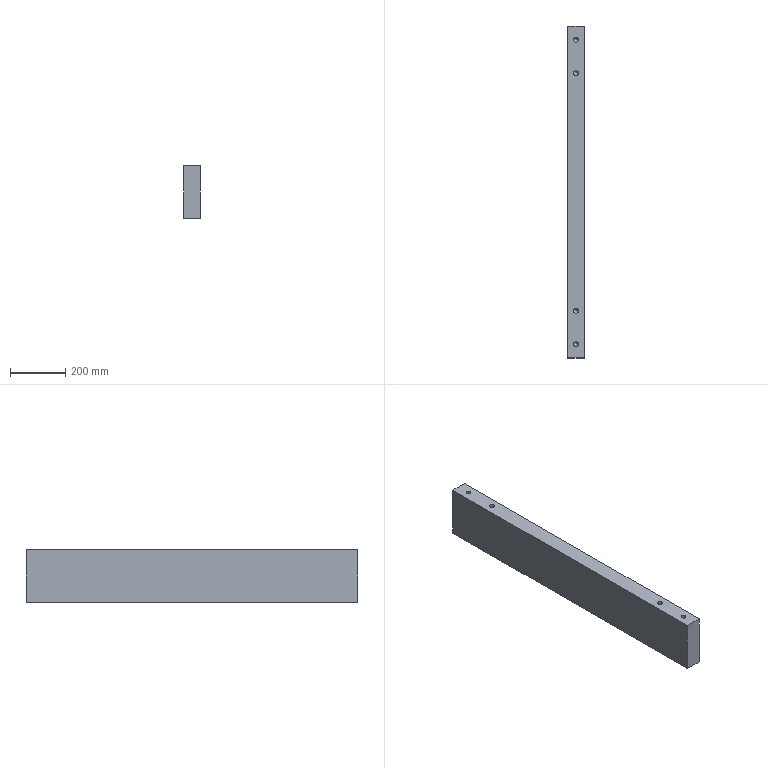Part | STEP file | lll_id4238_x_t | 1 solid | 22 faces | box 60 x 1200 x 190 mm | volume 13594949 mm3 | cylinder 8 | cone 8 | plane 6 | commonest cylinder face diameters 17.506 x7 17.505 x1
STEP:
#1=CARTESIAN_POINT('',(2996.188,-550.,-370.));
#2=VERTEX_POINT('',#1);
#3=CARTESIAN_POINT('',(2987.435,-550.,-370.));
#4=DIRECTION('',(0.,0.,1.));
#5=DIRECTION('',(1.,0.,0.));
#6=AXIS2_PLACEMENT_3D('',#3,#4,#5);
#7=CIRCLE('',#6,8.753);
#8=EDGE_CURVE('',#2,#2,#7,.T.);
#9=ORIENTED_EDGE('',*,*,#8,.T.);
#10=EDGE_LOOP('',(#9));
#11=FACE_BOUND('',#10,.T.);
#12=CARTESIAN_POINT('',(2996.188,550.,-370.));
#13=VERTEX_POINT('',#12);
#14=CARTESIAN_POINT('',(2987.435,550.,-370.));
#15=DIRECTION('',(0.,0.,1.));
#16=DIRECTION('',(1.,0.,0.));
#17=AXIS2_PLACEMENT_3D('',#14,#15,#16);
#18=CIRCLE('',#17,8.753);
#19=EDGE_CURVE('',#13,#13,#18,.T.);
#20=ORIENTED_EDGE('',*,*,#19,.T.);
#21=EDGE_LOOP('',(#20));
#22=FACE_BOUND('',#21,.T.);
#23=CARTESIAN_POINT('',(2957.435,600.,-370.));
#24=VERTEX_POINT('',#23);
#25=CARTESIAN_POINT('',(2957.435,-600.,-370.));
#26=VERTEX_POINT('',#25);
#27=CARTESIAN_POINT('',(2957.435,1.,-370.));
#28=DIRECTION('',(0.,-1.,0.));
#29=VECTOR('',#28,1.);
#30=LINE('',#27,#29);
#31=EDGE_CURVE('',#24,#26,#30,.T.);
#32=ORIENTED_EDGE('',*,*,#31,.F.);
#33=CARTESIAN_POINT('',(3017.435,600.,-370.));
#34=VERTEX_POINT('',#33);
#35=CARTESIAN_POINT('',(-952.565,600.,-370.));
#36=DIRECTION('',(1.,0.,0.));
#37=VECTOR('',#36,1.);
#38=LINE('',#35,#37);
#39=EDGE_CURVE('',#24,#34,#38,.T.);
#40=ORIENTED_EDGE('',*,*,#39,.T.);
#41=CARTESIAN_POINT('',(3017.435,-600.,-370.));
#42=VERTEX_POINT('',#41);
#43=CARTESIAN_POINT('',(3017.435,600.,-370.));
#44=DIRECTION('',(0.,-1.,0.));
#45=VECTOR('',#44,1.);
#46=LINE('',#43,#45);
#47=EDGE_CURVE('',#34,#42,#46,.T.);
#48=ORIENTED_EDGE('',*,*,#47,.T.);
#49=CARTESIAN_POINT('',(3017.435,-600.,-370.));
#50=DIRECTION('',(-1.,0.,0.));
#51=VECTOR('',#50,1.);
#52=LINE('',#49,#51);
#53=EDGE_CURVE('',#42,#26,#52,.T.);
#54=ORIENTED_EDGE('',*,*,#53,.T.);
#55=EDGE_LOOP('',(#32,#40,#48,#54));
#56=FACE_BOUND('',#55,.T.);
#57=CARTESIAN_POINT('',(2996.188,430.,-370.));
#58=VERTEX_POINT('',#57);
#59=CARTESIAN_POINT('',(2987.435,430.,-370.));
#60=DIRECTION('',(0.,0.,1.));
#61=DIRECTION('',(1.,0.,0.));
#62=AXIS2_PLACEMENT_3D('',#59,#60,#61);
#63=CIRCLE('',#62,8.753);
#64=EDGE_CURVE('',#58,#58,#63,.T.);
#65=ORIENTED_EDGE('',*,*,#64,.T.);
#66=EDGE_LOOP('',(#65));
#67=FACE_BOUND('',#66,.T.);
#68=CARTESIAN_POINT('',(2996.188,-430.,-370.));
#69=VERTEX_POINT('',#68);
#70=CARTESIAN_POINT('',(2987.435,-430.,-370.));
#71=DIRECTION('',(0.,0.,1.));
#72=DIRECTION('',(1.,0.,0.));
#73=AXIS2_PLACEMENT_3D('',#70,#71,#72);
#74=CIRCLE('',#73,8.752);
#75=EDGE_CURVE('',#69,#69,#74,.T.);
#76=ORIENTED_EDGE('',*,*,#75,.T.);
#77=EDGE_LOOP('',(#76));
#78=FACE_BOUND('',#77,.T.);
#79=CARTESIAN_POINT('',(5203.751,1.,-370.));
#80=DIRECTION('',(0.,0.,-1.));
#81=DIRECTION('',(-1.,0.,0.));
#82=AXIS2_PLACEMENT_3D('',#79,#80,#81);
#83=PLANE('',#82);
#84=ADVANCED_FACE('',(#11,#22,#56,#67,#78),#83,.T.);
#85=ORIENTED_EDGE('',*,*,#47,.F.);
#86=CARTESIAN_POINT('',(3017.435,600.,-180.));
#87=VERTEX_POINT('',#86);
#88=CARTESIAN_POINT('',(3017.435,600.,-182.5));
#89=DIRECTION('',(0.,0.,-1.));
#90=VECTOR('',#89,1.);
#91=LINE('',#88,#90);
#92=EDGE_CURVE('',#87,#34,#91,.T.);
#93=ORIENTED_EDGE('',*,*,#92,.F.);
#94=CARTESIAN_POINT('',(3017.435,-600.,-180.));
#95=VERTEX_POINT('',#94);
#96=CARTESIAN_POINT('',(3017.435,1.,-180.));
#97=DIRECTION('',(0.,-1.,0.));
#98=VECTOR('',#97,1.);
#99=LINE('',#96,#98);
#100=EDGE_CURVE('',#87,#95,#99,.T.);
#101=ORIENTED_EDGE('',*,*,#100,.T.);
#102=CARTESIAN_POINT('',(3017.435,-600.,-182.5));
#103=DIRECTION('',(0.,0.,-1.));
#104=VECTOR('',#103,1.);
#105=LINE('',#102,#104);
#106=EDGE_CURVE('',#95,#42,#105,.T.);
#107=ORIENTED_EDGE('',*,*,#106,.T.);
#108=EDGE_LOOP('',(#85,#93,#101,#107));
#109=FACE_OUTER_BOUND('',#108,.T.);
#110=CARTESIAN_POINT('',(3017.435,600.,-182.5));
#111=DIRECTION('',(1.,0.,0.));
#112=DIRECTION('',(0.,0.,-1.));
#113=AXIS2_PLACEMENT_3D('',#110,#111,#112);
#114=PLANE('',#113);
#115=ADVANCED_FACE('',(#109),#114,.T.);
#116=CARTESIAN_POINT('',(2957.435,-600.,-180.));
#117=VERTEX_POINT('',#116);
#118=CARTESIAN_POINT('',(2957.435,-600.,-182.5));
#119=DIRECTION('',(0.,0.,-1.));
#120=VECTOR('',#119,1.);
#121=LINE('',#118,#120);
#122=EDGE_CURVE('',#117,#26,#121,.T.);
#123=ORIENTED_EDGE('',*,*,#122,.T.);
#124=ORIENTED_EDGE('',*,*,#53,.F.);
#125=ORIENTED_EDGE('',*,*,#106,.F.);
#126=CARTESIAN_POINT('',(5203.751,-600.,-180.));
#127=DIRECTION('',(-1.,0.,0.));
#128=VECTOR('',#127,1.);
#129=LINE('',#126,#128);
#130=EDGE_CURVE('',#95,#117,#129,.T.);
#131=ORIENTED_EDGE('',*,*,#130,.T.);
#132=EDGE_LOOP('',(#123,#124,#125,#131));
#133=FACE_OUTER_BOUND('',#132,.T.);
#134=CARTESIAN_POINT('',(3017.435,-600.,-182.5));
#135=DIRECTION('',(0.,-1.,0.));
#136=DIRECTION('',(0.,0.,-1.));
#137=AXIS2_PLACEMENT_3D('',#134,#135,#136);
#138=PLANE('',#137);
#139=ADVANCED_FACE('',(#133),#138,.T.);
#140=CARTESIAN_POINT('',(2957.435,600.,-180.));
#141=VERTEX_POINT('',#140);
#142=CARTESIAN_POINT('',(2957.435,600.,-182.5));
#143=DIRECTION('',(0.,0.,1.));
#144=VECTOR('',#143,1.);
#145=LINE('',#142,#144);
#146=EDGE_CURVE('',#24,#141,#145,.T.);
#147=ORIENTED_EDGE('',*,*,#146,.T.);
#148=CARTESIAN_POINT('',(5203.751,600.,-180.));
#149=DIRECTION('',(1.,0.,0.));
#150=VECTOR('',#149,1.);
#151=LINE('',#148,#150);
#152=EDGE_CURVE('',#141,#87,#151,.T.);
#153=ORIENTED_EDGE('',*,*,#152,.T.);
#154=ORIENTED_EDGE('',*,*,#92,.T.);
#155=ORIENTED_EDGE('',*,*,#39,.F.);
#156=EDGE_LOOP('',(#147,#153,#154,#155));
#157=FACE_OUTER_BOUND('',#156,.T.);
#158=CARTESIAN_POINT('',(-952.565,600.,-182.5));
#159=DIRECTION('',(0.,1.,0.));
#160=DIRECTION('',(0.,0.,1.));
#161=AXIS2_PLACEMENT_3D('',#158,#159,#160);
#162=PLANE('',#161);
#163=ADVANCED_FACE('',(#157),#162,.T.);
#164=CARTESIAN_POINT('',(2996.188,-430.,-180.));
#165=VERTEX_POINT('',#164);
#166=CARTESIAN_POINT('',(2987.435,-430.,-180.));
#167=DIRECTION('',(0.,0.,-1.));
#168=DIRECTION('',(1.,0.,0.));
#169=AXIS2_PLACEMENT_3D('',#166,#167,#168);
#170=CIRCLE('',#169,8.753);
#171=EDGE_CURVE('',#165,#165,#170,.T.);
#172=ORIENTED_EDGE('',*,*,#171,.T.);
#173=EDGE_LOOP('',(#172));
#174=FACE_BOUND('',#173,.T.);
#175=CARTESIAN_POINT('',(2978.682,550.,-180.));
#176=VERTEX_POINT('',#175);
#177=CARTESIAN_POINT('',(2987.435,550.,-180.));
#178=DIRECTION('',(0.,0.,-1.));
#179=DIRECTION('',(-1.,0.,0.));
#180=AXIS2_PLACEMENT_3D('',#177,#178,#179);
#181=CIRCLE('',#180,8.753);
#182=EDGE_CURVE('',#176,#176,#181,.T.);
#183=ORIENTED_EDGE('',*,*,#182,.T.);
#184=EDGE_LOOP('',(#183));
#185=FACE_BOUND('',#184,.T.);
#186=CARTESIAN_POINT('',(2978.682,430.,-180.));
#187=VERTEX_POINT('',#186);
#188=CARTESIAN_POINT('',(2987.435,430.,-180.));
#189=DIRECTION('',(0.,0.,-1.));
#190=DIRECTION('',(-1.,0.,0.));
#191=AXIS2_PLACEMENT_3D('',#188,#189,#190);
#192=CIRCLE('',#191,8.753);
#193=EDGE_CURVE('',#187,#187,#192,.T.);
#194=ORIENTED_EDGE('',*,*,#193,.T.);
#195=EDGE_LOOP('',(#194));
#196=FACE_BOUND('',#195,.T.);
#197=CARTESIAN_POINT('',(2978.682,-550.,-180.));
#198=VERTEX_POINT('',#197);
#199=CARTESIAN_POINT('',(2987.435,-550.,-180.));
#200=DIRECTION('',(0.,0.,-1.));
#201=DIRECTION('',(-1.,0.,0.));
#202=AXIS2_PLACEMENT_3D('',#199,#200,#201);
#203=CIRCLE('',#202,8.753);
#204=EDGE_CURVE('',#198,#198,#203,.T.);
#205=ORIENTED_EDGE('',*,*,#204,.T.);
#206=EDGE_LOOP('',(#205));
#207=FACE_BOUND('',#206,.T.);
#208=ORIENTED_EDGE('',*,*,#152,.F.);
#209=CARTESIAN_POINT('',(2957.435,0.,-180.));
#210=DIRECTION('',(0.,1.,0.));
#211=VECTOR('',#210,1.);
#212=LINE('',#209,#211);
#213=EDGE_CURVE('',#117,#141,#212,.T.);
#214=ORIENTED_EDGE('',*,*,#213,.F.);
#215=ORIENTED_EDGE('',*,*,#130,.F.);
#216=ORIENTED_EDGE('',*,*,#100,.F.);
#217=EDGE_LOOP('',(#208,#214,#215,#216));
#218=FACE_BOUND('',#217,.T.);
#219=CARTESIAN_POINT('',(5203.751,1.,-180.));
#220=DIRECTION('',(0.,0.,-1.));
#221=DIRECTION('',(-1.,0.,0.));
#222=AXIS2_PLACEMENT_3D('',#219,#220,#221);
#223=PLANE('',#222);
#224=ADVANCED_FACE('',(#174,#185,#196,#207,#218),#223,.F.);
#225=ORIENTED_EDGE('',*,*,#146,.F.);
#226=ORIENTED_EDGE('',*,*,#31,.T.);
#227=ORIENTED_EDGE('',*,*,#122,.F.);
#228=ORIENTED_EDGE('',*,*,#213,.T.);
#229=EDGE_LOOP('',(#225,#226,#227,#228));
#230=FACE_OUTER_BOUND('',#229,.T.);
#231=CARTESIAN_POINT('',(2957.435,0.,-251.25));
#232=DIRECTION('',(1.,0.,0.));
#233=DIRECTION('',(0.,0.,-1.));
#234=AXIS2_PLACEMENT_3D('',#231,#232,#233);
#235=PLANE('',#234);
#236=ADVANCED_FACE('',(#230),#235,.F.);
#237=CARTESIAN_POINT('',(2978.682,-550.,-221.253));
#238=VERTEX_POINT('',#237);
#239=CARTESIAN_POINT('',(2987.435,-550.,-221.253));
#240=DIRECTION('',(0.,0.,-1.));
#241=DIRECTION('',(-1.,0.,0.));
#242=AXIS2_PLACEMENT_3D('',#239,#240,#241);
#243=CIRCLE('',#242,8.753);
#244=EDGE_CURVE('',#238,#238,#243,.T.);
#245=ORIENTED_EDGE('',*,*,#244,.T.);
#246=EDGE_LOOP('',(#245));
#247=FACE_BOUND('',#246,.T.);
#248=ORIENTED_EDGE('',*,*,#204,.F.);
#249=EDGE_LOOP('',(#248));
#250=FACE_BOUND('',#249,.T.);
#251=CARTESIAN_POINT('',(2987.435,-550.,-180.));
#252=DIRECTION('',(0.,0.,-1.));
#253=DIRECTION('',(1.,0.,0.));
#254=AXIS2_PLACEMENT_3D('',#251,#252,#253);
#255=CYLINDRICAL_SURFACE('',#254,8.753);
#256=ADVANCED_FACE('',(#247,#250),#255,.F.);
#257=CARTESIAN_POINT('',(2987.435,-550.,-230.006));
#258=VERTEX_POINT('',#257);
#259=VERTEX_LOOP('',#258);
#260=FACE_BOUND('',#259,.T.);
#261=ORIENTED_EDGE('',*,*,#244,.F.);
#262=EDGE_LOOP('',(#261));
#263=FACE_BOUND('',#262,.T.);
#264=CARTESIAN_POINT('',(2987.435,-550.,-221.253));
#265=DIRECTION('',(0.,0.,1.));
#266=DIRECTION('',(-1.,0.,0.));
#267=AXIS2_PLACEMENT_3D('',#264,#265,#266);
#268=CONICAL_SURFACE('',#267,8.753,45.);
#269=ADVANCED_FACE('',(#260,#263),#268,.F.);
#270=CARTESIAN_POINT('',(2978.682,430.,-221.253));
#271=VERTEX_POINT('',#270);
#272=CARTESIAN_POINT('',(2987.435,430.,-221.253));
#273=DIRECTION('',(0.,0.,-1.));
#274=DIRECTION('',(-1.,0.,0.));
#275=AXIS2_PLACEMENT_3D('',#272,#273,#274);
#276=CIRCLE('',#275,8.753);
#277=EDGE_CURVE('',#271,#271,#276,.T.);
#278=ORIENTED_EDGE('',*,*,#277,.T.);
#279=EDGE_LOOP('',(#278));
#280=FACE_BOUND('',#279,.T.);
#281=ORIENTED_EDGE('',*,*,#193,.F.);
#282=EDGE_LOOP('',(#281));
#283=FACE_BOUND('',#282,.T.);
#284=CARTESIAN_POINT('',(2987.435,430.,-180.));
#285=DIRECTION('',(0.,0.,-1.));
#286=DIRECTION('',(1.,0.,0.));
#287=AXIS2_PLACEMENT_3D('',#284,#285,#286);
#288=CYLINDRICAL_SURFACE('',#287,8.753);
#289=ADVANCED_FACE('',(#280,#283),#288,.F.);
#290=CARTESIAN_POINT('',(2987.435,430.,-230.006));
#291=VERTEX_POINT('',#290);
#292=VERTEX_LOOP('',#291);
#293=FACE_BOUND('',#292,.T.);
#294=ORIENTED_EDGE('',*,*,#277,.F.);
#295=EDGE_LOOP('',(#294));
#296=FACE_BOUND('',#295,.T.);
#297=CARTESIAN_POINT('',(2987.435,430.,-221.253));
#298=DIRECTION('',(0.,0.,1.));
#299=DIRECTION('',(-1.,0.,0.));
#300=AXIS2_PLACEMENT_3D('',#297,#298,#299);
#301=CONICAL_SURFACE('',#300,8.753,45.);
#302=ADVANCED_FACE('',(#293,#296),#301,.F.);
#303=CARTESIAN_POINT('',(2978.682,550.,-221.253));
#304=VERTEX_POINT('',#303);
#305=CARTESIAN_POINT('',(2987.435,550.,-221.253));
#306=DIRECTION('',(0.,0.,-1.));
#307=DIRECTION('',(-1.,0.,0.));
#308=AXIS2_PLACEMENT_3D('',#305,#306,#307);
#309=CIRCLE('',#308,8.753);
#310=EDGE_CURVE('',#304,#304,#309,.T.);
#311=ORIENTED_EDGE('',*,*,#310,.T.);
#312=EDGE_LOOP('',(#311));
#313=FACE_BOUND('',#312,.T.);
#314=ORIENTED_EDGE('',*,*,#182,.F.);
#315=EDGE_LOOP('',(#314));
#316=FACE_BOUND('',#315,.T.);
#317=CARTESIAN_POINT('',(2987.435,550.,-180.));
#318=DIRECTION('',(0.,0.,-1.));
#319=DIRECTION('',(1.,0.,0.));
#320=AXIS2_PLACEMENT_3D('',#317,#318,#319);
#321=CYLINDRICAL_SURFACE('',#320,8.753);
#322=ADVANCED_FACE('',(#313,#316),#321,.F.);
#323=CARTESIAN_POINT('',(2987.435,550.,-230.006));
#324=VERTEX_POINT('',#323);
#325=VERTEX_LOOP('',#324);
#326=FACE_BOUND('',#325,.T.);
#327=ORIENTED_EDGE('',*,*,#310,.F.);
#328=EDGE_LOOP('',(#327));
#329=FACE_BOUND('',#328,.T.);
#330=CARTESIAN_POINT('',(2987.435,550.,-221.253));
#331=DIRECTION('',(0.,0.,1.));
#332=DIRECTION('',(-1.,0.,0.));
#333=AXIS2_PLACEMENT_3D('',#330,#331,#332);
#334=CONICAL_SURFACE('',#333,8.753,45.);
#335=ADVANCED_FACE('',(#326,#329),#334,.F.);
#336=CARTESIAN_POINT('',(2996.188,550.,-328.747));
#337=VERTEX_POINT('',#336);
#338=CARTESIAN_POINT('',(2987.435,550.,-328.747));
#339=DIRECTION('',(0.,0.,1.));
#340=DIRECTION('',(1.,0.,0.));
#341=AXIS2_PLACEMENT_3D('',#338,#339,#340);
#342=CIRCLE('',#341,8.753);
#343=EDGE_CURVE('',#337,#337,#342,.T.);
#344=ORIENTED_EDGE('',*,*,#343,.T.);
#345=EDGE_LOOP('',(#344));
#346=FACE_BOUND('',#345,.T.);
#347=ORIENTED_EDGE('',*,*,#19,.F.);
#348=EDGE_LOOP('',(#347));
#349=FACE_BOUND('',#348,.T.);
#350=CARTESIAN_POINT('',(2987.435,550.,-370.));
#351=DIRECTION('',(0.,0.,1.));
#352=DIRECTION('',(-1.,0.,0.));
#353=AXIS2_PLACEMENT_3D('',#350,#351,#352);
#354=CYLINDRICAL_SURFACE('',#353,8.753);
#355=ADVANCED_FACE('',(#346,#349),#354,.F.);
#356=CARTESIAN_POINT('',(2987.435,550.,-319.994));
#357=VERTEX_POINT('',#356);
#358=VERTEX_LOOP('',#357);
#359=FACE_BOUND('',#358,.T.);
#360=ORIENTED_EDGE('',*,*,#343,.F.);
#361=EDGE_LOOP('',(#360));
#362=FACE_BOUND('',#361,.T.);
#363=CARTESIAN_POINT('',(2987.435,550.,-328.747));
#364=DIRECTION('',(0.,0.,-1.));
#365=DIRECTION('',(1.,0.,0.));
#366=AXIS2_PLACEMENT_3D('',#363,#364,#365);
#367=CONICAL_SURFACE('',#366,8.753,45.);
#368=ADVANCED_FACE('',(#359,#362),#367,.F.);
#369=CARTESIAN_POINT('',(2996.188,430.,-328.747));
#370=VERTEX_POINT('',#369);
#371=CARTESIAN_POINT('',(2987.435,430.,-328.747));
#372=DIRECTION('',(0.,0.,1.));
#373=DIRECTION('',(1.,0.,0.));
#374=AXIS2_PLACEMENT_3D('',#371,#372,#373);
#375=CIRCLE('',#374,8.753);
#376=EDGE_CURVE('',#370,#370,#375,.T.);
#377=ORIENTED_EDGE('',*,*,#376,.T.);
#378=EDGE_LOOP('',(#377));
#379=FACE_BOUND('',#378,.T.);
#380=ORIENTED_EDGE('',*,*,#64,.F.);
#381=EDGE_LOOP('',(#380));
#382=FACE_BOUND('',#381,.T.);
#383=CARTESIAN_POINT('',(2987.435,430.,-370.));
#384=DIRECTION('',(0.,0.,1.));
#385=DIRECTION('',(-1.,0.,0.));
#386=AXIS2_PLACEMENT_3D('',#383,#384,#385);
#387=CYLINDRICAL_SURFACE('',#386,8.753);
#388=ADVANCED_FACE('',(#379,#382),#387,.F.);
#389=CARTESIAN_POINT('',(2987.435,430.,-319.994));
#390=VERTEX_POINT('',#389);
#391=VERTEX_LOOP('',#390);
#392=FACE_BOUND('',#391,.T.);
#393=ORIENTED_EDGE('',*,*,#376,.F.);
#394=EDGE_LOOP('',(#393));
#395=FACE_BOUND('',#394,.T.);
#396=CARTESIAN_POINT('',(2987.435,430.,-328.747));
#397=DIRECTION('',(0.,0.,-1.));
#398=DIRECTION('',(1.,0.,0.));
#399=AXIS2_PLACEMENT_3D('',#396,#397,#398);
#400=CONICAL_SURFACE('',#399,8.753,45.);
#401=ADVANCED_FACE('',(#392,#395),#400,.F.);
#402=CARTESIAN_POINT('',(2996.188,-550.,-328.747));
#403=VERTEX_POINT('',#402);
#404=CARTESIAN_POINT('',(2987.435,-550.,-328.747));
#405=DIRECTION('',(0.,0.,1.));
#406=DIRECTION('',(1.,0.,0.));
#407=AXIS2_PLACEMENT_3D('',#404,#405,#406);
#408=CIRCLE('',#407,8.753);
#409=EDGE_CURVE('',#403,#403,#408,.T.);
#410=ORIENTED_EDGE('',*,*,#409,.T.);
#411=EDGE_LOOP('',(#410));
#412=FACE_BOUND('',#411,.T.);
#413=ORIENTED_EDGE('',*,*,#8,.F.);
#414=EDGE_LOOP('',(#413));
#415=FACE_BOUND('',#414,.T.);
#416=CARTESIAN_POINT('',(2987.435,-550.,-370.));
#417=DIRECTION('',(0.,0.,1.));
#418=DIRECTION('',(-1.,0.,0.));
#419=AXIS2_PLACEMENT_3D('',#416,#417,#418);
#420=CYLINDRICAL_SURFACE('',#419,8.753);
#421=ADVANCED_FACE('',(#412,#415),#420,.F.);
#422=CARTESIAN_POINT('',(2987.435,-550.,-319.994));
#423=VERTEX_POINT('',#422);
#424=VERTEX_LOOP('',#423);
#425=FACE_BOUND('',#424,.T.);
#426=ORIENTED_EDGE('',*,*,#409,.F.);
#427=EDGE_LOOP('',(#426));
#428=FACE_BOUND('',#427,.T.);
#429=CARTESIAN_POINT('',(2987.435,-550.,-328.747));
#430=DIRECTION('',(0.,0.,-1.));
#431=DIRECTION('',(1.,0.,0.));
#432=AXIS2_PLACEMENT_3D('',#429,#430,#431);
#433=CONICAL_SURFACE('',#432,8.753,45.);
#434=ADVANCED_FACE('',(#425,#428),#433,.F.);
#435=CARTESIAN_POINT('',(2978.682,-430.,-221.253));
#436=VERTEX_POINT('',#435);
#437=CARTESIAN_POINT('',(2987.435,-430.,-221.253));
#438=DIRECTION('',(0.,0.,-1.));
#439=DIRECTION('',(-1.,0.,0.));
#440=AXIS2_PLACEMENT_3D('',#437,#438,#439);
#441=CIRCLE('',#440,8.753);
#442=EDGE_CURVE('',#436,#436,#441,.T.);
#443=ORIENTED_EDGE('',*,*,#442,.T.);
#444=EDGE_LOOP('',(#443));
#445=FACE_BOUND('',#444,.T.);
#446=ORIENTED_EDGE('',*,*,#171,.F.);
#447=EDGE_LOOP('',(#446));
#448=FACE_BOUND('',#447,.T.);
#449=CARTESIAN_POINT('',(2987.435,-430.,-180.));
#450=DIRECTION('',(0.,0.,-1.));
#451=DIRECTION('',(-1.,0.,0.));
#452=AXIS2_PLACEMENT_3D('',#449,#450,#451);
#453=CYLINDRICAL_SURFACE('',#452,8.753);
#454=ADVANCED_FACE('',(#445,#448),#453,.F.);
#455=CARTESIAN_POINT('',(2987.435,-430.,-230.006));
#456=VERTEX_POINT('',#455);
#457=VERTEX_LOOP('',#456);
#458=FACE_BOUND('',#457,.T.);
#459=ORIENTED_EDGE('',*,*,#442,.F.);
#460=EDGE_LOOP('',(#459));
#461=FACE_BOUND('',#460,.T.);
#462=CARTESIAN_POINT('',(2987.435,-430.,-221.253));
#463=DIRECTION('',(0.,0.,1.));
#464=DIRECTION('',(-1.,0.,0.));
#465=AXIS2_PLACEMENT_3D('',#462,#463,#464);
#466=CONICAL_SURFACE('',#465,8.753,45.);
#467=ADVANCED_FACE('',(#458,#461),#466,.F.);
#468=CARTESIAN_POINT('',(2996.188,-430.,-328.747));
#469=VERTEX_POINT('',#468);
#470=CARTESIAN_POINT('',(2987.435,-430.,-328.747));
#471=DIRECTION('',(0.,0.,1.));
#472=DIRECTION('',(1.,0.,0.));
#473=AXIS2_PLACEMENT_3D('',#470,#471,#472);
#474=CIRCLE('',#473,8.752);
#475=EDGE_CURVE('',#469,#469,#474,.T.);
#476=ORIENTED_EDGE('',*,*,#475,.T.);
#477=EDGE_LOOP('',(#476));
#478=FACE_BOUND('',#477,.T.);
#479=ORIENTED_EDGE('',*,*,#75,.F.);
#480=EDGE_LOOP('',(#479));
#481=FACE_BOUND('',#480,.T.);
#482=CARTESIAN_POINT('',(2987.435,-430.,-370.));
#483=DIRECTION('',(0.,0.,1.));
#484=DIRECTION('',(-1.,0.,0.));
#485=AXIS2_PLACEMENT_3D('',#482,#483,#484);
#486=CYLINDRICAL_SURFACE('',#485,8.752);
#487=ADVANCED_FACE('',(#478,#481),#486,.F.);
#488=CARTESIAN_POINT('',(2987.435,-430.,-319.994));
#489=VERTEX_POINT('',#488);
#490=VERTEX_LOOP('',#489);
#491=FACE_BOUND('',#490,.T.);
#492=ORIENTED_EDGE('',*,*,#475,.F.);
#493=EDGE_LOOP('',(#492));
#494=FACE_BOUND('',#493,.T.);
#495=CARTESIAN_POINT('',(2987.435,-430.,-328.747));
#496=DIRECTION('',(0.,0.,-1.));
#497=DIRECTION('',(1.,0.,0.));
#498=AXIS2_PLACEMENT_3D('',#495,#496,#497);
#499=CONICAL_SURFACE('',#498,8.752,45.);
#500=ADVANCED_FACE('',(#491,#494),#499,.F.);
#501=CLOSED_SHELL('',(#84,#115,#139,#163,#224,#236,#256,#269,#289,#302,#322,#335,#355,#368,#388,#401,#421,#434,#454,#467,#487,#500));
#502=MANIFOLD_SOLID_BREP('',#501);
#503=(LENGTH_UNIT()NAMED_UNIT(*)SI_UNIT(.MILLI.,.METRE.));
#504=UNCERTAINTY_MEASURE_WITH_UNIT(LENGTH_MEASURE(0.00002),#503,'','');
#505=(NAMED_UNIT(*)PLANE_ANGLE_UNIT()SI_UNIT($,.RADIAN.));
#506=PLANE_ANGLE_MEASURE_WITH_UNIT(PLANE_ANGLE_MEASURE(0.01745),#505);
#507=DIMENSIONAL_EXPONENTS(0.,0.,0.,0.,0.,0.,0.);
#508=(CONVERSION_BASED_UNIT('DEGREE',#506)NAMED_UNIT(#507)PLANE_ANGLE_UNIT());
#509=(NAMED_UNIT(*)SI_UNIT($,.STERADIAN.)SOLID_ANGLE_UNIT());
#510=(GEOMETRIC_REPRESENTATION_CONTEXT(3)GLOBAL_UNCERTAINTY_ASSIGNED_CONTEXT((#504))GLOBAL_UNIT_ASSIGNED_CONTEXT((#503,#508,#509))REPRESENTATION_CONTEXT('',''));
#511=ADVANCED_BREP_SHAPE_REPRESENTATION('',(#502),#510);